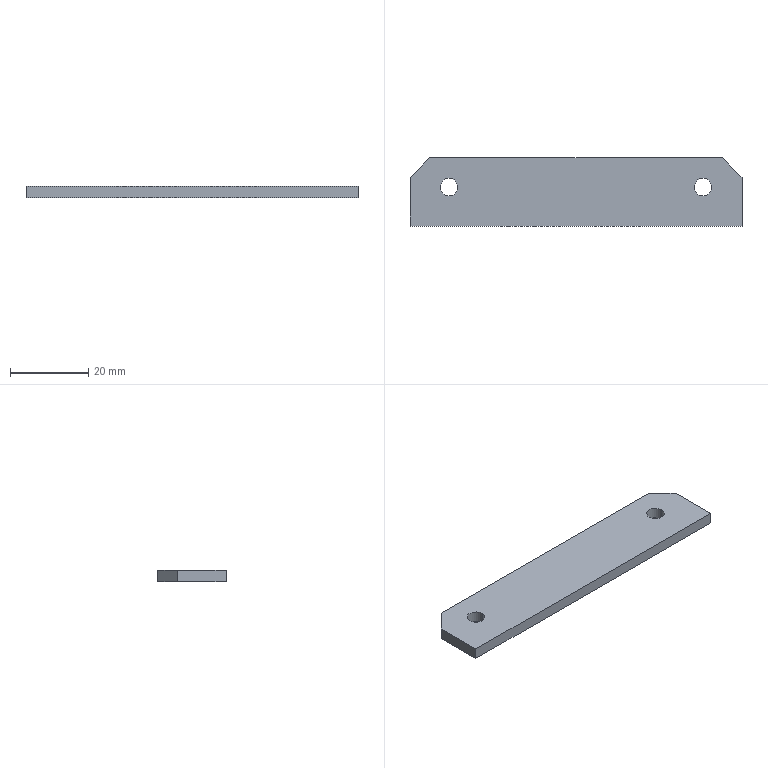Part | SolidWorks | features Cut 1, Extrusion 1 | 1 solid | 12 faces | box 85 x 17.5 x 3 mm | volume 4292 mm3 | plane 8 | cylinder 4 | commonest cylinder face diameters 4.5 x4
STEP:
#1=CARTESIAN_POINT('',(-638.75,119.2,-1.5));
#2=VERTEX_POINT('',#1);
#3=CARTESIAN_POINT('',(-634.25,119.2,-1.5));
#4=VERTEX_POINT('',#3);
#5=CARTESIAN_POINT('',(-636.5,119.2,-1.5));
#6=DIRECTION('',(0.,0.,1.));
#7=DIRECTION('',(1.,0.,0.));
#8=AXIS2_PLACEMENT_3D('',#5,#6,#7);
#9=CIRCLE('',#8,2.25);
#10=EDGE_CURVE('',#2,#4,#9,.T.);
#11=ORIENTED_EDGE('',*,*,#10,.F.);
#12=CARTESIAN_POINT('',(-638.75,119.2,1.5));
#13=VERTEX_POINT('',#12);
#14=CARTESIAN_POINT('',(-638.75,119.2,-1.5));
#15=DIRECTION('',(0.,0.,1.));
#16=VECTOR('',#15,1000.);
#17=LINE('',#14,#16);
#18=EDGE_CURVE('',#2,#13,#17,.T.);
#19=ORIENTED_EDGE('',*,*,#18,.T.);
#20=CARTESIAN_POINT('',(-634.25,119.2,1.5));
#21=VERTEX_POINT('',#20);
#22=CARTESIAN_POINT('',(-636.5,119.2,1.5));
#23=DIRECTION('',(0.,0.,1.));
#24=DIRECTION('',(1.,0.,0.));
#25=AXIS2_PLACEMENT_3D('',#22,#23,#24);
#26=CIRCLE('',#25,2.25);
#27=EDGE_CURVE('',#13,#21,#26,.T.);
#28=ORIENTED_EDGE('',*,*,#27,.T.);
#29=CARTESIAN_POINT('',(-634.25,119.2,-1.5));
#30=DIRECTION('',(0.,0.,1.));
#31=VECTOR('',#30,1000.);
#32=LINE('',#29,#31);
#33=EDGE_CURVE('',#4,#21,#32,.T.);
#34=ORIENTED_EDGE('',*,*,#33,.F.);
#35=EDGE_LOOP('',(#11,#19,#28,#34));
#36=FACE_OUTER_BOUND('',#35,.T.);
#37=CARTESIAN_POINT('',(-636.5,119.2,-1.5));
#38=DIRECTION('',(0.,0.,1.));
#39=DIRECTION('',(1.,0.,0.));
#40=AXIS2_PLACEMENT_3D('',#37,#38,#39);
#41=CYLINDRICAL_SURFACE('',#40,2.25);
#42=ADVANCED_FACE('',(#36),#41,.F.);
#43=CARTESIAN_POINT('',(-573.75,119.2,-1.5));
#44=VERTEX_POINT('',#43);
#45=CARTESIAN_POINT('',(-569.25,119.2,-1.5));
#46=VERTEX_POINT('',#45);
#47=CARTESIAN_POINT('',(-571.5,119.2,-1.5));
#48=DIRECTION('',(0.,0.,1.));
#49=DIRECTION('',(1.,0.,0.));
#50=AXIS2_PLACEMENT_3D('',#47,#48,#49);
#51=CIRCLE('',#50,2.25);
#52=EDGE_CURVE('',#44,#46,#51,.T.);
#53=ORIENTED_EDGE('',*,*,#52,.F.);
#54=CARTESIAN_POINT('',(-573.75,119.2,1.5));
#55=VERTEX_POINT('',#54);
#56=CARTESIAN_POINT('',(-573.75,119.2,-1.5));
#57=DIRECTION('',(0.,0.,1.));
#58=VECTOR('',#57,1000.);
#59=LINE('',#56,#58);
#60=EDGE_CURVE('',#44,#55,#59,.T.);
#61=ORIENTED_EDGE('',*,*,#60,.T.);
#62=CARTESIAN_POINT('',(-569.25,119.2,1.5));
#63=VERTEX_POINT('',#62);
#64=CARTESIAN_POINT('',(-571.5,119.2,1.5));
#65=DIRECTION('',(0.,0.,1.));
#66=DIRECTION('',(1.,0.,0.));
#67=AXIS2_PLACEMENT_3D('',#64,#65,#66);
#68=CIRCLE('',#67,2.25);
#69=EDGE_CURVE('',#55,#63,#68,.T.);
#70=ORIENTED_EDGE('',*,*,#69,.T.);
#71=CARTESIAN_POINT('',(-569.25,119.2,-1.5));
#72=DIRECTION('',(0.,0.,1.));
#73=VECTOR('',#72,1000.);
#74=LINE('',#71,#73);
#75=EDGE_CURVE('',#46,#63,#74,.T.);
#76=ORIENTED_EDGE('',*,*,#75,.F.);
#77=EDGE_LOOP('',(#53,#61,#70,#76));
#78=FACE_OUTER_BOUND('',#77,.T.);
#79=CARTESIAN_POINT('',(-571.5,119.2,-1.5));
#80=DIRECTION('',(0.,0.,1.));
#81=DIRECTION('',(1.,0.,0.));
#82=AXIS2_PLACEMENT_3D('',#79,#80,#81);
#83=CYLINDRICAL_SURFACE('',#82,2.25);
#84=ADVANCED_FACE('',(#78),#83,.F.);
#85=CARTESIAN_POINT('',(-646.5,121.7,-1.5));
#86=VERTEX_POINT('',#85);
#87=CARTESIAN_POINT('',(-646.5,109.2,-1.5));
#88=VERTEX_POINT('',#87);
#89=CARTESIAN_POINT('',(-646.5,109.2,-1.5));
#90=DIRECTION('',(0.,-1.,0.));
#91=VECTOR('',#90,1000.);
#92=LINE('',#89,#91);
#93=EDGE_CURVE('',#86,#88,#92,.T.);
#94=ORIENTED_EDGE('',*,*,#93,.T.);
#95=CARTESIAN_POINT('',(-646.5,109.2,1.5));
#96=VERTEX_POINT('',#95);
#97=CARTESIAN_POINT('',(-646.5,109.2,1.5));
#98=DIRECTION('',(0.,0.,-1.));
#99=VECTOR('',#98,1000.);
#100=LINE('',#97,#99);
#101=EDGE_CURVE('',#96,#88,#100,.T.);
#102=ORIENTED_EDGE('',*,*,#101,.F.);
#103=CARTESIAN_POINT('',(-646.5,121.7,1.5));
#104=VERTEX_POINT('',#103);
#105=CARTESIAN_POINT('',(-646.5,109.2,1.5));
#106=DIRECTION('',(0.,-1.,0.));
#107=VECTOR('',#106,1000.);
#108=LINE('',#105,#107);
#109=EDGE_CURVE('',#104,#96,#108,.T.);
#110=ORIENTED_EDGE('',*,*,#109,.F.);
#111=CARTESIAN_POINT('',(-646.5,121.7,1.5));
#112=DIRECTION('',(0.,0.,-1.));
#113=VECTOR('',#112,1000.);
#114=LINE('',#111,#113);
#115=EDGE_CURVE('',#104,#86,#114,.T.);
#116=ORIENTED_EDGE('',*,*,#115,.T.);
#117=EDGE_LOOP('',(#94,#102,#110,#116));
#118=FACE_OUTER_BOUND('',#117,.T.);
#119=CARTESIAN_POINT('',(-646.5,109.2,1.5));
#120=DIRECTION('',(1.,0.,0.));
#121=DIRECTION('',(0.,0.,-1.));
#122=AXIS2_PLACEMENT_3D('',#119,#120,#121);
#123=PLANE('',#122);
#124=ADVANCED_FACE('',(#118),#123,.F.);
#125=CARTESIAN_POINT('',(-561.5,109.2,-1.5));
#126=VERTEX_POINT('',#125);
#127=CARTESIAN_POINT('',(-646.5,109.2,-1.5));
#128=DIRECTION('',(1.,0.,0.));
#129=VECTOR('',#128,1000.);
#130=LINE('',#127,#129);
#131=EDGE_CURVE('',#88,#126,#130,.T.);
#132=ORIENTED_EDGE('',*,*,#131,.T.);
#133=CARTESIAN_POINT('',(-561.5,109.2,1.5));
#134=VERTEX_POINT('',#133);
#135=CARTESIAN_POINT('',(-561.5,109.2,1.5));
#136=DIRECTION('',(0.,0.,-1.));
#137=VECTOR('',#136,1000.);
#138=LINE('',#135,#137);
#139=EDGE_CURVE('',#134,#126,#138,.T.);
#140=ORIENTED_EDGE('',*,*,#139,.F.);
#141=CARTESIAN_POINT('',(-646.5,109.2,1.5));
#142=DIRECTION('',(1.,0.,0.));
#143=VECTOR('',#142,1000.);
#144=LINE('',#141,#143);
#145=EDGE_CURVE('',#96,#134,#144,.T.);
#146=ORIENTED_EDGE('',*,*,#145,.F.);
#147=ORIENTED_EDGE('',*,*,#101,.T.);
#148=EDGE_LOOP('',(#132,#140,#146,#147));
#149=FACE_OUTER_BOUND('',#148,.T.);
#150=CARTESIAN_POINT('',(-646.5,109.2,1.5));
#151=DIRECTION('',(0.,1.,0.));
#152=DIRECTION('',(0.,0.,1.));
#153=AXIS2_PLACEMENT_3D('',#150,#151,#152);
#154=PLANE('',#153);
#155=ADVANCED_FACE('',(#149),#154,.F.);
#156=CARTESIAN_POINT('',(-561.5,121.7,-1.5));
#157=VERTEX_POINT('',#156);
#158=CARTESIAN_POINT('',(-561.5,109.2,-1.5));
#159=DIRECTION('',(0.,1.,0.));
#160=VECTOR('',#159,1000.);
#161=LINE('',#158,#160);
#162=EDGE_CURVE('',#126,#157,#161,.T.);
#163=ORIENTED_EDGE('',*,*,#162,.T.);
#164=CARTESIAN_POINT('',(-561.5,121.7,1.5));
#165=VERTEX_POINT('',#164);
#166=CARTESIAN_POINT('',(-561.5,121.7,1.5));
#167=DIRECTION('',(0.,0.,-1.));
#168=VECTOR('',#167,1000.);
#169=LINE('',#166,#168);
#170=EDGE_CURVE('',#165,#157,#169,.T.);
#171=ORIENTED_EDGE('',*,*,#170,.F.);
#172=CARTESIAN_POINT('',(-561.5,109.2,1.5));
#173=DIRECTION('',(0.,1.,0.));
#174=VECTOR('',#173,1000.);
#175=LINE('',#172,#174);
#176=EDGE_CURVE('',#134,#165,#175,.T.);
#177=ORIENTED_EDGE('',*,*,#176,.F.);
#178=ORIENTED_EDGE('',*,*,#139,.T.);
#179=EDGE_LOOP('',(#163,#171,#177,#178));
#180=FACE_OUTER_BOUND('',#179,.T.);
#181=CARTESIAN_POINT('',(-561.5,109.2,1.5));
#182=DIRECTION('',(-1.,0.,0.));
#183=DIRECTION('',(0.,0.,1.));
#184=AXIS2_PLACEMENT_3D('',#181,#182,#183);
#185=PLANE('',#184);
#186=ADVANCED_FACE('',(#180),#185,.F.);
#187=CARTESIAN_POINT('',(-566.5,126.7,-1.5));
#188=VERTEX_POINT('',#187);
#189=CARTESIAN_POINT('',(-566.5,126.7,-1.5));
#190=DIRECTION('',(-0.7071,0.7071,0.));
#191=VECTOR('',#190,1000.);
#192=LINE('',#189,#191);
#193=EDGE_CURVE('',#157,#188,#192,.T.);
#194=ORIENTED_EDGE('',*,*,#193,.T.);
#195=CARTESIAN_POINT('',(-566.5,126.7,1.5));
#196=VERTEX_POINT('',#195);
#197=CARTESIAN_POINT('',(-566.5,126.7,1.5));
#198=DIRECTION('',(0.,0.,-1.));
#199=VECTOR('',#198,1000.);
#200=LINE('',#197,#199);
#201=EDGE_CURVE('',#196,#188,#200,.T.);
#202=ORIENTED_EDGE('',*,*,#201,.F.);
#203=CARTESIAN_POINT('',(-566.5,126.7,1.5));
#204=DIRECTION('',(-0.7071,0.7071,0.));
#205=VECTOR('',#204,1000.);
#206=LINE('',#203,#205);
#207=EDGE_CURVE('',#165,#196,#206,.T.);
#208=ORIENTED_EDGE('',*,*,#207,.F.);
#209=ORIENTED_EDGE('',*,*,#170,.T.);
#210=EDGE_LOOP('',(#194,#202,#208,#209));
#211=FACE_OUTER_BOUND('',#210,.T.);
#212=CARTESIAN_POINT('',(-566.5,126.7,1.5));
#213=DIRECTION('',(-0.7071,-0.7071,0.));
#214=DIRECTION('',(0.7071,-0.7071,0.));
#215=AXIS2_PLACEMENT_3D('',#212,#213,#214);
#216=PLANE('',#215);
#217=ADVANCED_FACE('',(#211),#216,.F.);
#218=CARTESIAN_POINT('',(-641.5,126.7,-1.5));
#219=VERTEX_POINT('',#218);
#220=CARTESIAN_POINT('',(-641.5,126.7,-1.5));
#221=DIRECTION('',(-1.,0.,0.));
#222=VECTOR('',#221,1000.);
#223=LINE('',#220,#222);
#224=EDGE_CURVE('',#188,#219,#223,.T.);
#225=ORIENTED_EDGE('',*,*,#224,.T.);
#226=CARTESIAN_POINT('',(-641.5,126.7,1.5));
#227=VERTEX_POINT('',#226);
#228=CARTESIAN_POINT('',(-641.5,126.7,1.5));
#229=DIRECTION('',(0.,0.,-1.));
#230=VECTOR('',#229,1000.);
#231=LINE('',#228,#230);
#232=EDGE_CURVE('',#227,#219,#231,.T.);
#233=ORIENTED_EDGE('',*,*,#232,.F.);
#234=CARTESIAN_POINT('',(-641.5,126.7,1.5));
#235=DIRECTION('',(-1.,0.,0.));
#236=VECTOR('',#235,1000.);
#237=LINE('',#234,#236);
#238=EDGE_CURVE('',#196,#227,#237,.T.);
#239=ORIENTED_EDGE('',*,*,#238,.F.);
#240=ORIENTED_EDGE('',*,*,#201,.T.);
#241=EDGE_LOOP('',(#225,#233,#239,#240));
#242=FACE_OUTER_BOUND('',#241,.T.);
#243=CARTESIAN_POINT('',(-641.5,126.7,1.5));
#244=DIRECTION('',(0.,-1.,0.));
#245=DIRECTION('',(1.,0.,0.));
#246=AXIS2_PLACEMENT_3D('',#243,#244,#245);
#247=PLANE('',#246);
#248=ADVANCED_FACE('',(#242),#247,.F.);
#249=CARTESIAN_POINT('',(-646.5,121.7,-1.5));
#250=DIRECTION('',(-0.7071,-0.7071,0.));
#251=VECTOR('',#250,1000.);
#252=LINE('',#249,#251);
#253=EDGE_CURVE('',#219,#86,#252,.T.);
#254=ORIENTED_EDGE('',*,*,#253,.T.);
#255=ORIENTED_EDGE('',*,*,#115,.F.);
#256=CARTESIAN_POINT('',(-646.5,121.7,1.5));
#257=DIRECTION('',(-0.7071,-0.7071,0.));
#258=VECTOR('',#257,1000.);
#259=LINE('',#256,#258);
#260=EDGE_CURVE('',#227,#104,#259,.T.);
#261=ORIENTED_EDGE('',*,*,#260,.F.);
#262=ORIENTED_EDGE('',*,*,#232,.T.);
#263=EDGE_LOOP('',(#254,#255,#261,#262));
#264=FACE_OUTER_BOUND('',#263,.T.);
#265=CARTESIAN_POINT('',(-646.5,121.7,1.5));
#266=DIRECTION('',(0.7071,-0.7071,0.));
#267=DIRECTION('',(0.7071,0.7071,0.));
#268=AXIS2_PLACEMENT_3D('',#265,#266,#267);
#269=PLANE('',#268);
#270=ADVANCED_FACE('',(#264),#269,.F.);
#271=CARTESIAN_POINT('',(-636.5,119.2,1.5));
#272=DIRECTION('',(0.,0.,1.));
#273=DIRECTION('',(1.,0.,0.));
#274=AXIS2_PLACEMENT_3D('',#271,#272,#273);
#275=CIRCLE('',#274,2.25);
#276=EDGE_CURVE('',#21,#13,#275,.T.);
#277=ORIENTED_EDGE('',*,*,#276,.F.);
#278=ORIENTED_EDGE('',*,*,#27,.F.);
#279=EDGE_LOOP('',(#277,#278));
#280=FACE_BOUND('',#279,.T.);
#281=CARTESIAN_POINT('',(-571.5,119.2,1.5));
#282=DIRECTION('',(0.,0.,1.));
#283=DIRECTION('',(1.,0.,0.));
#284=AXIS2_PLACEMENT_3D('',#281,#282,#283);
#285=CIRCLE('',#284,2.25);
#286=EDGE_CURVE('',#63,#55,#285,.T.);
#287=ORIENTED_EDGE('',*,*,#286,.F.);
#288=ORIENTED_EDGE('',*,*,#69,.F.);
#289=EDGE_LOOP('',(#287,#288));
#290=FACE_BOUND('',#289,.T.);
#291=ORIENTED_EDGE('',*,*,#109,.T.);
#292=ORIENTED_EDGE('',*,*,#145,.T.);
#293=ORIENTED_EDGE('',*,*,#176,.T.);
#294=ORIENTED_EDGE('',*,*,#207,.T.);
#295=ORIENTED_EDGE('',*,*,#238,.T.);
#296=ORIENTED_EDGE('',*,*,#260,.T.);
#297=EDGE_LOOP('',(#291,#292,#293,#294,#295,#296));
#298=FACE_OUTER_BOUND('',#297,.T.);
#299=CARTESIAN_POINT('',(0.,0.,1.5));
#300=DIRECTION('',(0.,0.,-1.));
#301=DIRECTION('',(-1.,0.,0.));
#302=AXIS2_PLACEMENT_3D('',#299,#300,#301);
#303=PLANE('',#302);
#304=ADVANCED_FACE('',(#280,#290,#298),#303,.F.);
#305=CARTESIAN_POINT('',(-636.5,119.2,-1.5));
#306=DIRECTION('',(0.,0.,1.));
#307=DIRECTION('',(1.,0.,0.));
#308=AXIS2_PLACEMENT_3D('',#305,#306,#307);
#309=CIRCLE('',#308,2.25);
#310=EDGE_CURVE('',#4,#2,#309,.T.);
#311=ORIENTED_EDGE('',*,*,#310,.T.);
#312=ORIENTED_EDGE('',*,*,#10,.T.);
#313=EDGE_LOOP('',(#311,#312));
#314=FACE_BOUND('',#313,.T.);
#315=CARTESIAN_POINT('',(-571.5,119.2,-1.5));
#316=DIRECTION('',(0.,0.,1.));
#317=DIRECTION('',(1.,0.,0.));
#318=AXIS2_PLACEMENT_3D('',#315,#316,#317);
#319=CIRCLE('',#318,2.25);
#320=EDGE_CURVE('',#46,#44,#319,.T.);
#321=ORIENTED_EDGE('',*,*,#320,.T.);
#322=ORIENTED_EDGE('',*,*,#52,.T.);
#323=EDGE_LOOP('',(#321,#322));
#324=FACE_BOUND('',#323,.T.);
#325=ORIENTED_EDGE('',*,*,#93,.F.);
#326=ORIENTED_EDGE('',*,*,#253,.F.);
#327=ORIENTED_EDGE('',*,*,#224,.F.);
#328=ORIENTED_EDGE('',*,*,#193,.F.);
#329=ORIENTED_EDGE('',*,*,#162,.F.);
#330=ORIENTED_EDGE('',*,*,#131,.F.);
#331=EDGE_LOOP('',(#325,#326,#327,#328,#329,#330));
#332=FACE_OUTER_BOUND('',#331,.T.);
#333=CARTESIAN_POINT('',(0.,0.,-1.5));
#334=DIRECTION('',(0.,0.,-1.));
#335=DIRECTION('',(-1.,0.,0.));
#336=AXIS2_PLACEMENT_3D('',#333,#334,#335);
#337=PLANE('',#336);
#338=ADVANCED_FACE('',(#314,#324,#332),#337,.T.);
#339=ORIENTED_EDGE('',*,*,#60,.F.);
#340=ORIENTED_EDGE('',*,*,#320,.F.);
#341=ORIENTED_EDGE('',*,*,#75,.T.);
#342=ORIENTED_EDGE('',*,*,#286,.T.);
#343=EDGE_LOOP('',(#339,#340,#341,#342));
#344=FACE_OUTER_BOUND('',#343,.T.);
#345=CARTESIAN_POINT('',(-571.5,119.2,-1.5));
#346=DIRECTION('',(0.,0.,1.));
#347=DIRECTION('',(1.,0.,0.));
#348=AXIS2_PLACEMENT_3D('',#345,#346,#347);
#349=CYLINDRICAL_SURFACE('',#348,2.25);
#350=ADVANCED_FACE('',(#344),#349,.F.);
#351=ORIENTED_EDGE('',*,*,#18,.F.);
#352=ORIENTED_EDGE('',*,*,#310,.F.);
#353=ORIENTED_EDGE('',*,*,#33,.T.);
#354=ORIENTED_EDGE('',*,*,#276,.T.);
#355=EDGE_LOOP('',(#351,#352,#353,#354));
#356=FACE_OUTER_BOUND('',#355,.T.);
#357=CARTESIAN_POINT('',(-636.5,119.2,-1.5));
#358=DIRECTION('',(0.,0.,1.));
#359=DIRECTION('',(1.,0.,0.));
#360=AXIS2_PLACEMENT_3D('',#357,#358,#359);
#361=CYLINDRICAL_SURFACE('',#360,2.25);
#362=ADVANCED_FACE('',(#356),#361,.F.);
#363=CLOSED_SHELL('',(#42,#84,#124,#155,#186,#217,#248,#270,#304,#338,#350,#362));
#364=MANIFOLD_SOLID_BREP('',#363);
#365=CARTESIAN_POINT('',(0.,0.,0.));
#366=DIRECTION('',(0.,0.,1.));
#367=DIRECTION('',(1.,0.,0.));
#368=AXIS2_PLACEMENT_3D('',#365,#366,#367);
#369=(LENGTH_UNIT()NAMED_UNIT(*)SI_UNIT(.MILLI.,.METRE.));
#370=UNCERTAINTY_MEASURE_WITH_UNIT(LENGTH_MEASURE(0.00001),#369,'','');
#371=(NAMED_UNIT(*)PLANE_ANGLE_UNIT()SI_UNIT($,.RADIAN.));
#372=(NAMED_UNIT(*)SI_UNIT($,.STERADIAN.)SOLID_ANGLE_UNIT());
#373=(GEOMETRIC_REPRESENTATION_CONTEXT(3)GLOBAL_UNCERTAINTY_ASSIGNED_CONTEXT((#370))GLOBAL_UNIT_ASSIGNED_CONTEXT((#369,#371,#372))REPRESENTATION_CONTEXT('',''));
#374=ADVANCED_BREP_SHAPE_REPRESENTATION('',(#364,#368),#373);